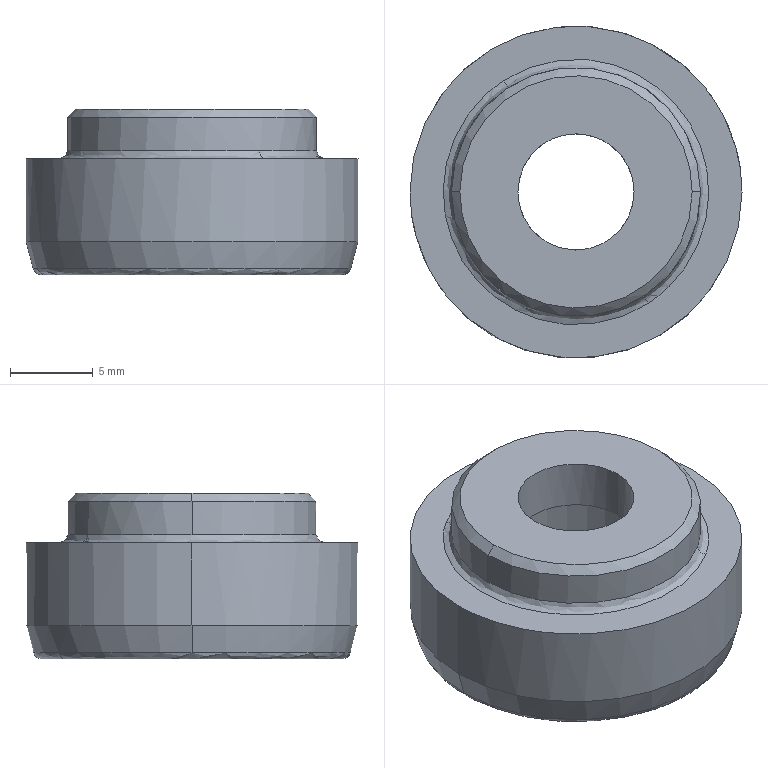Part | STEP file | _1971-A | 1 solid | 20 faces | box 20 x 20 x 10 mm | volume 1911 mm3 | cylinder 8 | spline 4 | cone 4 | plane 4 | commonest cylinder face diameters 7 x2 11 x2 15 x2 20 x2